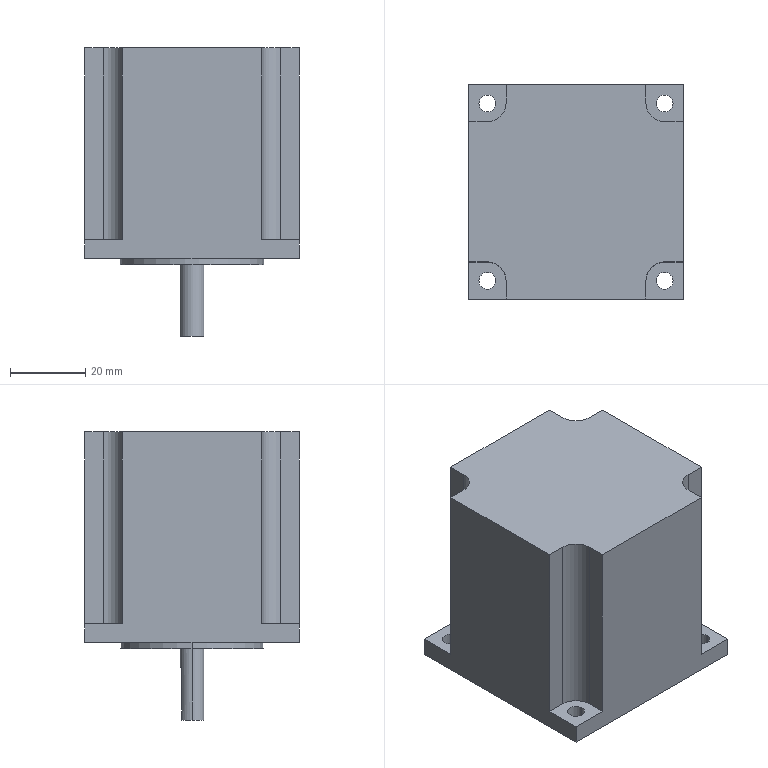Part | STEP file | Stepping motor YK57HB56-03A | 1 solid | 38 faces | box 57 x 57 x 76.6 mm | volume 165114 mm3 | plane 22 | cylinder 16 | commonest cylinder face diameters 4.5 x8 9.9 x4 6.35 x2 38.1 x2
STEP:
#1=CARTESIAN_POINT('',(-3.175,0.,-20.6));
#2=VERTEX_POINT('',#1);
#3=CARTESIAN_POINT('',(-1.71,2.675,-20.6));
#4=VERTEX_POINT('',#3);
#5=CARTESIAN_POINT('',(0.,0.,-20.6));
#6=DIRECTION('',(0.,0.,-1.));
#7=DIRECTION('',(-1.,0.,0.));
#8=AXIS2_PLACEMENT_3D('',#5,#6,#7);
#9=CIRCLE('',#8,3.175);
#10=EDGE_CURVE('',#2,#4,#9,.T.);
#11=ORIENTED_EDGE('',*,*,#10,.F.);
#12=CARTESIAN_POINT('',(-3.175,0.,-1.6));
#13=VERTEX_POINT('',#12);
#14=CARTESIAN_POINT('',(-3.175,0.,-20.6));
#15=DIRECTION('',(0.,0.,1.));
#16=VECTOR('',#15,1000.);
#17=LINE('',#14,#16);
#18=EDGE_CURVE('',#2,#13,#17,.T.);
#19=ORIENTED_EDGE('',*,*,#18,.T.);
#20=CARTESIAN_POINT('',(3.175,0.,-1.6));
#21=VERTEX_POINT('',#20);
#22=CARTESIAN_POINT('',(0.,0.,-1.6));
#23=DIRECTION('',(0.,0.,-1.));
#24=DIRECTION('',(-1.,0.,0.));
#25=AXIS2_PLACEMENT_3D('',#22,#23,#24);
#26=CIRCLE('',#25,3.175);
#27=EDGE_CURVE('',#13,#21,#26,.T.);
#28=ORIENTED_EDGE('',*,*,#27,.T.);
#29=CARTESIAN_POINT('',(3.175,0.,-20.6));
#30=VERTEX_POINT('',#29);
#31=CARTESIAN_POINT('',(3.175,0.,-20.6));
#32=DIRECTION('',(0.,0.,1.));
#33=VECTOR('',#32,1000.);
#34=LINE('',#31,#33);
#35=EDGE_CURVE('',#30,#21,#34,.T.);
#36=ORIENTED_EDGE('',*,*,#35,.F.);
#37=CARTESIAN_POINT('',(1.71,2.675,-20.6));
#38=VERTEX_POINT('',#37);
#39=CARTESIAN_POINT('',(0.,0.,-20.6));
#40=DIRECTION('',(0.,0.,-1.));
#41=DIRECTION('',(-1.,0.,0.));
#42=AXIS2_PLACEMENT_3D('',#39,#40,#41);
#43=CIRCLE('',#42,3.175);
#44=EDGE_CURVE('',#38,#30,#43,.T.);
#45=ORIENTED_EDGE('',*,*,#44,.F.);
#46=CARTESIAN_POINT('',(1.71,2.675,-6.6));
#47=VERTEX_POINT('',#46);
#48=CARTESIAN_POINT('',(1.71,2.675,-6.6));
#49=DIRECTION('',(0.,0.,-1.));
#50=VECTOR('',#49,1000.);
#51=LINE('',#48,#50);
#52=EDGE_CURVE('',#47,#38,#51,.T.);
#53=ORIENTED_EDGE('',*,*,#52,.F.);
#54=CARTESIAN_POINT('',(-1.71,2.675,-6.6));
#55=VERTEX_POINT('',#54);
#56=CARTESIAN_POINT('',(0.,0.,-6.6));
#57=DIRECTION('',(0.,0.,-1.));
#58=DIRECTION('',(-1.,0.,0.));
#59=AXIS2_PLACEMENT_3D('',#56,#57,#58);
#60=CIRCLE('',#59,3.175);
#61=EDGE_CURVE('',#55,#47,#60,.T.);
#62=ORIENTED_EDGE('',*,*,#61,.F.);
#63=CARTESIAN_POINT('',(-1.71,2.675,-6.6));
#64=DIRECTION('',(0.,0.,-1.));
#65=VECTOR('',#64,1000.);
#66=LINE('',#63,#65);
#67=EDGE_CURVE('',#55,#4,#66,.T.);
#68=ORIENTED_EDGE('',*,*,#67,.T.);
#69=EDGE_LOOP('',(#11,#19,#28,#36,#45,#53,#62,#68));
#70=FACE_OUTER_BOUND('',#69,.T.);
#71=CARTESIAN_POINT('',(0.,0.,-20.6));
#72=DIRECTION('',(0.,0.,1.));
#73=DIRECTION('',(1.,0.,0.));
#74=AXIS2_PLACEMENT_3D('',#71,#72,#73);
#75=CYLINDRICAL_SURFACE('',#74,3.175);
#76=ADVANCED_FACE('',(#70),#75,.T.);
#77=CARTESIAN_POINT('',(-19.05,0.,-1.6));
#78=VERTEX_POINT('',#77);
#79=CARTESIAN_POINT('',(19.05,0.,-1.6));
#80=VERTEX_POINT('',#79);
#81=CARTESIAN_POINT('',(0.,0.,-1.6));
#82=DIRECTION('',(0.,0.,-1.));
#83=DIRECTION('',(-1.,0.,0.));
#84=AXIS2_PLACEMENT_3D('',#81,#82,#83);
#85=CIRCLE('',#84,19.05);
#86=EDGE_CURVE('',#78,#80,#85,.T.);
#87=ORIENTED_EDGE('',*,*,#86,.F.);
#88=CARTESIAN_POINT('',(-19.05,0.,0.));
#89=VERTEX_POINT('',#88);
#90=CARTESIAN_POINT('',(-19.05,0.,-1.6));
#91=DIRECTION('',(0.,0.,1.));
#92=VECTOR('',#91,1000.);
#93=LINE('',#90,#92);
#94=EDGE_CURVE('',#78,#89,#93,.T.);
#95=ORIENTED_EDGE('',*,*,#94,.T.);
#96=CARTESIAN_POINT('',(19.05,0.,0.));
#97=VERTEX_POINT('',#96);
#98=CARTESIAN_POINT('',(0.,0.,0.));
#99=DIRECTION('',(0.,0.,-1.));
#100=DIRECTION('',(1.,0.,0.));
#101=AXIS2_PLACEMENT_3D('',#98,#99,#100);
#102=CIRCLE('',#101,19.05);
#103=EDGE_CURVE('',#89,#97,#102,.T.);
#104=ORIENTED_EDGE('',*,*,#103,.T.);
#105=CARTESIAN_POINT('',(19.05,0.,-1.6));
#106=DIRECTION('',(0.,0.,1.));
#107=VECTOR('',#106,1000.);
#108=LINE('',#105,#107);
#109=EDGE_CURVE('',#80,#97,#108,.T.);
#110=ORIENTED_EDGE('',*,*,#109,.F.);
#111=EDGE_LOOP('',(#87,#95,#104,#110));
#112=FACE_OUTER_BOUND('',#111,.T.);
#113=CARTESIAN_POINT('',(0.,0.,-1.6));
#114=DIRECTION('',(0.,0.,1.));
#115=DIRECTION('',(1.,0.,0.));
#116=AXIS2_PLACEMENT_3D('',#113,#114,#115);
#117=CYLINDRICAL_SURFACE('',#116,19.05);
#118=ADVANCED_FACE('',(#112),#117,.T.);
#119=CARTESIAN_POINT('',(21.3,-23.55,5.));
#120=VERTEX_POINT('',#119);
#121=CARTESIAN_POINT('',(25.8,-23.55,5.));
#122=VERTEX_POINT('',#121);
#123=CARTESIAN_POINT('',(23.55,-23.55,5.));
#124=DIRECTION('',(0.,0.,1.));
#125=DIRECTION('',(-1.,0.,0.));
#126=AXIS2_PLACEMENT_3D('',#123,#124,#125);
#127=CIRCLE('',#126,2.25);
#128=EDGE_CURVE('',#120,#122,#127,.T.);
#129=ORIENTED_EDGE('',*,*,#128,.T.);
#130=CARTESIAN_POINT('',(25.8,-23.55,0.));
#131=VERTEX_POINT('',#130);
#132=CARTESIAN_POINT('',(25.8,-23.55,0.));
#133=DIRECTION('',(0.,0.,-1.));
#134=VECTOR('',#133,1000.);
#135=LINE('',#132,#134);
#136=EDGE_CURVE('',#122,#131,#135,.T.);
#137=ORIENTED_EDGE('',*,*,#136,.T.);
#138=CARTESIAN_POINT('',(21.3,-23.55,0.));
#139=VERTEX_POINT('',#138);
#140=CARTESIAN_POINT('',(23.55,-23.55,0.));
#141=DIRECTION('',(0.,0.,-1.));
#142=DIRECTION('',(-1.,0.,0.));
#143=AXIS2_PLACEMENT_3D('',#140,#141,#142);
#144=CIRCLE('',#143,2.25);
#145=EDGE_CURVE('',#131,#139,#144,.T.);
#146=ORIENTED_EDGE('',*,*,#145,.T.);
#147=CARTESIAN_POINT('',(21.3,-23.55,0.));
#148=DIRECTION('',(0.,0.,-1.));
#149=VECTOR('',#148,1000.);
#150=LINE('',#147,#149);
#151=EDGE_CURVE('',#120,#139,#150,.T.);
#152=ORIENTED_EDGE('',*,*,#151,.F.);
#153=EDGE_LOOP('',(#129,#137,#146,#152));
#154=FACE_OUTER_BOUND('',#153,.T.);
#155=CARTESIAN_POINT('',(23.55,-23.55,0.));
#156=DIRECTION('',(0.,0.,-1.));
#157=DIRECTION('',(-1.,0.,0.));
#158=AXIS2_PLACEMENT_3D('',#155,#156,#157);
#159=CYLINDRICAL_SURFACE('',#158,2.25);
#160=ADVANCED_FACE('',(#154),#159,.F.);
#161=CARTESIAN_POINT('',(-25.8,-23.55,5.));
#162=VERTEX_POINT('',#161);
#163=CARTESIAN_POINT('',(-21.3,-23.55,5.));
#164=VERTEX_POINT('',#163);
#165=CARTESIAN_POINT('',(-23.55,-23.55,5.));
#166=DIRECTION('',(0.,0.,1.));
#167=DIRECTION('',(-1.,0.,0.));
#168=AXIS2_PLACEMENT_3D('',#165,#166,#167);
#169=CIRCLE('',#168,2.25);
#170=EDGE_CURVE('',#162,#164,#169,.T.);
#171=ORIENTED_EDGE('',*,*,#170,.T.);
#172=CARTESIAN_POINT('',(-21.3,-23.55,0.));
#173=VERTEX_POINT('',#172);
#174=CARTESIAN_POINT('',(-21.3,-23.55,0.));
#175=DIRECTION('',(0.,0.,-1.));
#176=VECTOR('',#175,1000.);
#177=LINE('',#174,#176);
#178=EDGE_CURVE('',#164,#173,#177,.T.);
#179=ORIENTED_EDGE('',*,*,#178,.T.);
#180=CARTESIAN_POINT('',(-25.8,-23.55,0.));
#181=VERTEX_POINT('',#180);
#182=CARTESIAN_POINT('',(-23.55,-23.55,0.));
#183=DIRECTION('',(0.,0.,-1.));
#184=DIRECTION('',(-1.,0.,0.));
#185=AXIS2_PLACEMENT_3D('',#182,#183,#184);
#186=CIRCLE('',#185,2.25);
#187=EDGE_CURVE('',#173,#181,#186,.T.);
#188=ORIENTED_EDGE('',*,*,#187,.T.);
#189=CARTESIAN_POINT('',(-25.8,-23.55,0.));
#190=DIRECTION('',(0.,0.,-1.));
#191=VECTOR('',#190,1000.);
#192=LINE('',#189,#191);
#193=EDGE_CURVE('',#162,#181,#192,.T.);
#194=ORIENTED_EDGE('',*,*,#193,.F.);
#195=EDGE_LOOP('',(#171,#179,#188,#194));
#196=FACE_OUTER_BOUND('',#195,.T.);
#197=CARTESIAN_POINT('',(-23.55,-23.55,0.));
#198=DIRECTION('',(0.,0.,-1.));
#199=DIRECTION('',(-1.,0.,0.));
#200=AXIS2_PLACEMENT_3D('',#197,#198,#199);
#201=CYLINDRICAL_SURFACE('',#200,2.25);
#202=ADVANCED_FACE('',(#196),#201,.F.);
#203=CARTESIAN_POINT('',(-25.8,23.55,5.));
#204=VERTEX_POINT('',#203);
#205=CARTESIAN_POINT('',(-21.3,23.55,5.));
#206=VERTEX_POINT('',#205);
#207=CARTESIAN_POINT('',(-23.55,23.55,5.));
#208=DIRECTION('',(0.,0.,1.));
#209=DIRECTION('',(-1.,0.,0.));
#210=AXIS2_PLACEMENT_3D('',#207,#208,#209);
#211=CIRCLE('',#210,2.25);
#212=EDGE_CURVE('',#204,#206,#211,.T.);
#213=ORIENTED_EDGE('',*,*,#212,.T.);
#214=CARTESIAN_POINT('',(-21.3,23.55,0.));
#215=VERTEX_POINT('',#214);
#216=CARTESIAN_POINT('',(-21.3,23.55,0.));
#217=DIRECTION('',(0.,0.,-1.));
#218=VECTOR('',#217,1000.);
#219=LINE('',#216,#218);
#220=EDGE_CURVE('',#206,#215,#219,.T.);
#221=ORIENTED_EDGE('',*,*,#220,.T.);
#222=CARTESIAN_POINT('',(-25.8,23.55,0.));
#223=VERTEX_POINT('',#222);
#224=CARTESIAN_POINT('',(-23.55,23.55,0.));
#225=DIRECTION('',(0.,0.,-1.));
#226=DIRECTION('',(-1.,0.,0.));
#227=AXIS2_PLACEMENT_3D('',#224,#225,#226);
#228=CIRCLE('',#227,2.25);
#229=EDGE_CURVE('',#215,#223,#228,.T.);
#230=ORIENTED_EDGE('',*,*,#229,.T.);
#231=CARTESIAN_POINT('',(-25.8,23.55,0.));
#232=DIRECTION('',(0.,0.,-1.));
#233=VECTOR('',#232,1000.);
#234=LINE('',#231,#233);
#235=EDGE_CURVE('',#204,#223,#234,.T.);
#236=ORIENTED_EDGE('',*,*,#235,.F.);
#237=EDGE_LOOP('',(#213,#221,#230,#236));
#238=FACE_OUTER_BOUND('',#237,.T.);
#239=CARTESIAN_POINT('',(-23.55,23.55,0.));
#240=DIRECTION('',(0.,0.,-1.));
#241=DIRECTION('',(-1.,0.,0.));
#242=AXIS2_PLACEMENT_3D('',#239,#240,#241);
#243=CYLINDRICAL_SURFACE('',#242,2.25);
#244=ADVANCED_FACE('',(#238),#243,.F.);
#245=CARTESIAN_POINT('',(21.3,23.55,5.));
#246=VERTEX_POINT('',#245);
#247=CARTESIAN_POINT('',(25.8,23.55,5.));
#248=VERTEX_POINT('',#247);
#249=CARTESIAN_POINT('',(23.55,23.55,5.));
#250=DIRECTION('',(0.,0.,1.));
#251=DIRECTION('',(-1.,0.,0.));
#252=AXIS2_PLACEMENT_3D('',#249,#250,#251);
#253=CIRCLE('',#252,2.25);
#254=EDGE_CURVE('',#246,#248,#253,.T.);
#255=ORIENTED_EDGE('',*,*,#254,.T.);
#256=CARTESIAN_POINT('',(25.8,23.55,0.));
#257=VERTEX_POINT('',#256);
#258=CARTESIAN_POINT('',(25.8,23.55,0.));
#259=DIRECTION('',(0.,0.,-1.));
#260=VECTOR('',#259,1000.);
#261=LINE('',#258,#260);
#262=EDGE_CURVE('',#248,#257,#261,.T.);
#263=ORIENTED_EDGE('',*,*,#262,.T.);
#264=CARTESIAN_POINT('',(21.3,23.55,0.));
#265=VERTEX_POINT('',#264);
#266=CARTESIAN_POINT('',(23.55,23.55,0.));
#267=DIRECTION('',(0.,0.,-1.));
#268=DIRECTION('',(-1.,0.,0.));
#269=AXIS2_PLACEMENT_3D('',#266,#267,#268);
#270=CIRCLE('',#269,2.25);
#271=EDGE_CURVE('',#257,#265,#270,.T.);
#272=ORIENTED_EDGE('',*,*,#271,.T.);
#273=CARTESIAN_POINT('',(21.3,23.55,0.));
#274=DIRECTION('',(0.,0.,-1.));
#275=VECTOR('',#274,1000.);
#276=LINE('',#273,#275);
#277=EDGE_CURVE('',#246,#265,#276,.T.);
#278=ORIENTED_EDGE('',*,*,#277,.F.);
#279=EDGE_LOOP('',(#255,#263,#272,#278));
#280=FACE_OUTER_BOUND('',#279,.T.);
#281=CARTESIAN_POINT('',(23.55,23.55,0.));
#282=DIRECTION('',(0.,0.,-1.));
#283=DIRECTION('',(-1.,0.,0.));
#284=AXIS2_PLACEMENT_3D('',#281,#282,#283);
#285=CYLINDRICAL_SURFACE('',#284,2.25);
#286=ADVANCED_FACE('',(#280),#285,.F.);
#287=CARTESIAN_POINT('',(-28.5,28.5,0.));
#288=VERTEX_POINT('',#287);
#289=CARTESIAN_POINT('',(-28.5,-28.5,0.));
#290=VERTEX_POINT('',#289);
#291=CARTESIAN_POINT('',(-28.5,-28.5,0.));
#292=DIRECTION('',(0.,-1.,0.));
#293=VECTOR('',#292,1000.);
#294=LINE('',#291,#293);
#295=EDGE_CURVE('',#288,#290,#294,.T.);
#296=ORIENTED_EDGE('',*,*,#295,.F.);
#297=CARTESIAN_POINT('',(28.5,28.5,0.));
#298=VERTEX_POINT('',#297);
#299=CARTESIAN_POINT('',(28.5,28.5,0.));
#300=DIRECTION('',(-1.,0.,0.));
#301=VECTOR('',#300,1000.);
#302=LINE('',#299,#301);
#303=EDGE_CURVE('',#298,#288,#302,.T.);
#304=ORIENTED_EDGE('',*,*,#303,.F.);
#305=CARTESIAN_POINT('',(28.5,-28.5,0.));
#306=VERTEX_POINT('',#305);
#307=CARTESIAN_POINT('',(28.5,-28.5,0.));
#308=DIRECTION('',(0.,1.,0.));
#309=VECTOR('',#308,1000.);
#310=LINE('',#307,#309);
#311=EDGE_CURVE('',#306,#298,#310,.T.);
#312=ORIENTED_EDGE('',*,*,#311,.F.);
#313=CARTESIAN_POINT('',(28.5,-28.5,0.));
#314=DIRECTION('',(1.,0.,0.));
#315=VECTOR('',#314,1000.);
#316=LINE('',#313,#315);
#317=EDGE_CURVE('',#290,#306,#316,.T.);
#318=ORIENTED_EDGE('',*,*,#317,.F.);
#319=EDGE_LOOP('',(#296,#304,#312,#318));
#320=FACE_OUTER_BOUND('',#319,.T.);
#321=CARTESIAN_POINT('',(23.55,23.55,0.));
#322=DIRECTION('',(0.,0.,-1.));
#323=DIRECTION('',(-1.,0.,0.));
#324=AXIS2_PLACEMENT_3D('',#321,#322,#323);
#325=CIRCLE('',#324,2.25);
#326=EDGE_CURVE('',#265,#257,#325,.T.);
#327=ORIENTED_EDGE('',*,*,#326,.F.);
#328=ORIENTED_EDGE('',*,*,#271,.F.);
#329=EDGE_LOOP('',(#327,#328));
#330=FACE_BOUND('',#329,.T.);
#331=CARTESIAN_POINT('',(-23.55,23.55,0.));
#332=DIRECTION('',(0.,0.,-1.));
#333=DIRECTION('',(-1.,0.,0.));
#334=AXIS2_PLACEMENT_3D('',#331,#332,#333);
#335=CIRCLE('',#334,2.25);
#336=EDGE_CURVE('',#223,#215,#335,.T.);
#337=ORIENTED_EDGE('',*,*,#336,.F.);
#338=ORIENTED_EDGE('',*,*,#229,.F.);
#339=EDGE_LOOP('',(#337,#338));
#340=FACE_BOUND('',#339,.T.);
#341=CARTESIAN_POINT('',(-23.55,-23.55,0.));
#342=DIRECTION('',(0.,0.,-1.));
#343=DIRECTION('',(-1.,0.,0.));
#344=AXIS2_PLACEMENT_3D('',#341,#342,#343);
#345=CIRCLE('',#344,2.25);
#346=EDGE_CURVE('',#181,#173,#345,.T.);
#347=ORIENTED_EDGE('',*,*,#346,.F.);
#348=ORIENTED_EDGE('',*,*,#187,.F.);
#349=EDGE_LOOP('',(#347,#348));
#350=FACE_BOUND('',#349,.T.);
#351=CARTESIAN_POINT('',(23.55,-23.55,0.));
#352=DIRECTION('',(0.,0.,-1.));
#353=DIRECTION('',(-1.,0.,0.));
#354=AXIS2_PLACEMENT_3D('',#351,#352,#353);
#355=CIRCLE('',#354,2.25);
#356=EDGE_CURVE('',#139,#131,#355,.T.);
#357=ORIENTED_EDGE('',*,*,#356,.F.);
#358=ORIENTED_EDGE('',*,*,#145,.F.);
#359=EDGE_LOOP('',(#357,#358));
#360=FACE_BOUND('',#359,.T.);
#361=CARTESIAN_POINT('',(0.,0.,0.));
#362=DIRECTION('',(0.,0.,-1.));
#363=DIRECTION('',(1.,0.,0.));
#364=AXIS2_PLACEMENT_3D('',#361,#362,#363);
#365=CIRCLE('',#364,19.05);
#366=EDGE_CURVE('',#97,#89,#365,.T.);
#367=ORIENTED_EDGE('',*,*,#366,.F.);
#368=ORIENTED_EDGE('',*,*,#103,.F.);
#369=EDGE_LOOP('',(#367,#368));
#370=FACE_BOUND('',#369,.T.);
#371=CARTESIAN_POINT('',(-28.5,28.5,0.));
#372=DIRECTION('',(0.,0.,1.));
#373=DIRECTION('',(1.,0.,0.));
#374=AXIS2_PLACEMENT_3D('',#371,#372,#373);
#375=PLANE('',#374);
#376=ADVANCED_FACE('',(#320,#330,#340,#350,#360,#370),#375,.F.);
#377=CARTESIAN_POINT('',(-28.5,-28.5,5.));
#378=VERTEX_POINT('',#377);
#379=CARTESIAN_POINT('',(-28.5,-18.6,5.));
#380=VERTEX_POINT('',#379);
#381=CARTESIAN_POINT('',(-28.5,-18.6,5.));
#382=DIRECTION('',(0.,1.,0.));
#383=VECTOR('',#382,1000.);
#384=LINE('',#381,#383);
#385=EDGE_CURVE('',#378,#380,#384,.T.);
#386=ORIENTED_EDGE('',*,*,#385,.T.);
#387=CARTESIAN_POINT('',(-28.5,-18.6,56.));
#388=VERTEX_POINT('',#387);
#389=CARTESIAN_POINT('',(-28.5,-18.6,56.));
#390=DIRECTION('',(0.,0.,-1.));
#391=VECTOR('',#390,1000.);
#392=LINE('',#389,#391);
#393=EDGE_CURVE('',#388,#380,#392,.T.);
#394=ORIENTED_EDGE('',*,*,#393,.F.);
#395=CARTESIAN_POINT('',(-28.5,18.6,56.));
#396=VERTEX_POINT('',#395);
#397=CARTESIAN_POINT('',(-28.5,-28.5,56.));
#398=DIRECTION('',(0.,-1.,0.));
#399=VECTOR('',#398,1000.);
#400=LINE('',#397,#399);
#401=EDGE_CURVE('',#396,#388,#400,.T.);
#402=ORIENTED_EDGE('',*,*,#401,.F.);
#403=CARTESIAN_POINT('',(-28.5,18.6,5.));
#404=VERTEX_POINT('',#403);
#405=CARTESIAN_POINT('',(-28.5,18.6,56.));
#406=DIRECTION('',(0.,0.,-1.));
#407=VECTOR('',#406,1000.);
#408=LINE('',#405,#407);
#409=EDGE_CURVE('',#396,#404,#408,.T.);
#410=ORIENTED_EDGE('',*,*,#409,.T.);
#411=CARTESIAN_POINT('',(-28.5,28.5,5.));
#412=VERTEX_POINT('',#411);
#413=CARTESIAN_POINT('',(-28.5,28.5,5.));
#414=DIRECTION('',(0.,1.,0.));
#415=VECTOR('',#414,1000.);
#416=LINE('',#413,#415);
#417=EDGE_CURVE('',#404,#412,#416,.T.);
#418=ORIENTED_EDGE('',*,*,#417,.T.);
#419=CARTESIAN_POINT('',(-28.5,28.5,56.));
#420=DIRECTION('',(0.,0.,-1.));
#421=VECTOR('',#420,1000.);
#422=LINE('',#419,#421);
#423=EDGE_CURVE('',#412,#288,#422,.T.);
#424=ORIENTED_EDGE('',*,*,#423,.T.);
#425=ORIENTED_EDGE('',*,*,#295,.T.);
#426=CARTESIAN_POINT('',(-28.5,-28.5,56.));
#427=DIRECTION('',(0.,0.,-1.));
#428=VECTOR('',#427,1000.);
#429=LINE('',#426,#428);
#430=EDGE_CURVE('',#378,#290,#429,.T.);
#431=ORIENTED_EDGE('',*,*,#430,.F.);
#432=EDGE_LOOP('',(#386,#394,#402,#410,#418,#424,#425,#431));
#433=FACE_OUTER_BOUND('',#432,.T.);
#434=CARTESIAN_POINT('',(-28.5,-28.5,56.));
#435=DIRECTION('',(1.,0.,0.));
#436=DIRECTION('',(0.,0.,-1.));
#437=AXIS2_PLACEMENT_3D('',#434,#435,#436);
#438=PLANE('',#437);
#439=ADVANCED_FACE('',(#433),#438,.F.);
#440=CARTESIAN_POINT('',(28.5,-28.5,5.));
#441=VERTEX_POINT('',#440);
#442=CARTESIAN_POINT('',(18.6,-28.5,5.));
#443=VERTEX_POINT('',#442);
#444=CARTESIAN_POINT('',(18.6,-28.5,5.));
#445=DIRECTION('',(-1.,0.,0.));
#446=VECTOR('',#445,1000.);
#447=LINE('',#444,#446);
#448=EDGE_CURVE('',#441,#443,#447,.T.);
#449=ORIENTED_EDGE('',*,*,#448,.T.);
#450=CARTESIAN_POINT('',(18.6,-28.5,56.));
#451=VERTEX_POINT('',#450);
#452=CARTESIAN_POINT('',(18.6,-28.5,56.));
#453=DIRECTION('',(0.,0.,-1.));
#454=VECTOR('',#453,1000.);
#455=LINE('',#452,#454);
#456=EDGE_CURVE('',#451,#443,#455,.T.);
#457=ORIENTED_EDGE('',*,*,#456,.F.);
#458=CARTESIAN_POINT('',(-18.6,-28.5,56.));
#459=VERTEX_POINT('',#458);
#460=CARTESIAN_POINT('',(28.5,-28.5,56.));
#461=DIRECTION('',(1.,0.,0.));
#462=VECTOR('',#461,1000.);
#463=LINE('',#460,#462);
#464=EDGE_CURVE('',#459,#451,#463,.T.);
#465=ORIENTED_EDGE('',*,*,#464,.F.);
#466=CARTESIAN_POINT('',(-18.6,-28.5,5.));
#467=VERTEX_POINT('',#466);
#468=CARTESIAN_POINT('',(-18.6,-28.5,56.));
#469=DIRECTION('',(0.,0.,-1.));
#470=VECTOR('',#469,1000.);
#471=LINE('',#468,#470);
#472=EDGE_CURVE('',#459,#467,#471,.T.);
#473=ORIENTED_EDGE('',*,*,#472,.T.);
#474=CARTESIAN_POINT('',(-28.5,-28.5,5.));
#475=DIRECTION('',(-1.,0.,0.));
#476=VECTOR('',#475,1000.);
#477=LINE('',#474,#476);
#478=EDGE_CURVE('',#467,#378,#477,.T.);
#479=ORIENTED_EDGE('',*,*,#478,.T.);
#480=ORIENTED_EDGE('',*,*,#430,.T.);
#481=ORIENTED_EDGE('',*,*,#317,.T.);
#482=CARTESIAN_POINT('',(28.5,-28.5,56.));
#483=DIRECTION('',(0.,0.,-1.));
#484=VECTOR('',#483,1000.);
#485=LINE('',#482,#484);
#486=EDGE_CURVE('',#441,#306,#485,.T.);
#487=ORIENTED_EDGE('',*,*,#486,.F.);
#488=EDGE_LOOP('',(#449,#457,#465,#473,#479,#480,#481,#487));
#489=FACE_OUTER_BOUND('',#488,.T.);
#490=CARTESIAN_POINT('',(28.5,-28.5,56.));
#491=DIRECTION('',(0.,1.,0.));
#492=DIRECTION('',(-1.,0.,0.));
#493=AXIS2_PLACEMENT_3D('',#490,#491,#492);
#494=PLANE('',#493);
#495=ADVANCED_FACE('',(#489),#494,.F.);
#496=CARTESIAN_POINT('',(28.5,-18.6,56.));
#497=VERTEX_POINT('',#496);
#498=CARTESIAN_POINT('',(28.5,18.6,56.));
#499=VERTEX_POINT('',#498);
#500=CARTESIAN_POINT('',(28.5,-28.5,56.));
#501=DIRECTION('',(0.,1.,0.));
#502=VECTOR('',#501,1000.);
#503=LINE('',#500,#502);
#504=EDGE_CURVE('',#497,#499,#503,.T.);
#505=ORIENTED_EDGE('',*,*,#504,.F.);
#506=CARTESIAN_POINT('',(28.5,-18.6,5.));
#507=VERTEX_POINT('',#506);
#508=CARTESIAN_POINT('',(28.5,-18.6,56.));
#509=DIRECTION('',(0.,0.,-1.));
#510=VECTOR('',#509,1000.);
#511=LINE('',#508,#510);
#512=EDGE_CURVE('',#497,#507,#511,.T.);
#513=ORIENTED_EDGE('',*,*,#512,.T.);
#514=CARTESIAN_POINT('',(28.5,-28.5,5.));
#515=DIRECTION('',(0.,-1.,0.));
#516=VECTOR('',#515,1000.);
#517=LINE('',#514,#516);
#518=EDGE_CURVE('',#507,#441,#517,.T.);
#519=ORIENTED_EDGE('',*,*,#518,.T.);
#520=ORIENTED_EDGE('',*,*,#486,.T.);
#521=ORIENTED_EDGE('',*,*,#311,.T.);
#522=CARTESIAN_POINT('',(28.5,28.5,5.));
#523=VERTEX_POINT('',#522);
#524=CARTESIAN_POINT('',(28.5,28.5,56.));
#525=DIRECTION('',(0.,0.,-1.));
#526=VECTOR('',#525,1000.);
#527=LINE('',#524,#526);
#528=EDGE_CURVE('',#523,#298,#527,.T.);
#529=ORIENTED_EDGE('',*,*,#528,.F.);
#530=CARTESIAN_POINT('',(28.5,18.6,5.));
#531=VERTEX_POINT('',#530);
#532=CARTESIAN_POINT('',(28.5,18.6,5.));
#533=DIRECTION('',(0.,-1.,0.));
#534=VECTOR('',#533,1000.);
#535=LINE('',#532,#534);
#536=EDGE_CURVE('',#523,#531,#535,.T.);
#537=ORIENTED_EDGE('',*,*,#536,.T.);
#538=CARTESIAN_POINT('',(28.5,18.6,56.));
#539=DIRECTION('',(0.,0.,-1.));
#540=VECTOR('',#539,1000.);
#541=LINE('',#538,#540);
#542=EDGE_CURVE('',#499,#531,#541,.T.);
#543=ORIENTED_EDGE('',*,*,#542,.F.);
#544=EDGE_LOOP('',(#505,#513,#519,#520,#521,#529,#537,#543));
#545=FACE_OUTER_BOUND('',#544,.T.);
#546=CARTESIAN_POINT('',(28.5,-28.5,56.));
#547=DIRECTION('',(-1.,0.,0.));
#548=DIRECTION('',(0.,0.,1.));
#549=AXIS2_PLACEMENT_3D('',#546,#547,#548);
#550=PLANE('',#549);
#551=ADVANCED_FACE('',(#545),#550,.F.);
#552=CARTESIAN_POINT('',(-18.6,28.5,5.));
#553=VERTEX_POINT('',#552);
#554=CARTESIAN_POINT('',(-18.6,28.5,5.));
#555=DIRECTION('',(1.,0.,0.));
#556=VECTOR('',#555,1000.);
#557=LINE('',#554,#556);
#558=EDGE_CURVE('',#412,#553,#557,.T.);
#559=ORIENTED_EDGE('',*,*,#558,.T.);
#560=CARTESIAN_POINT('',(-18.6,28.5,56.));
#561=VERTEX_POINT('',#560);
#562=CARTESIAN_POINT('',(-18.6,28.5,56.));
#563=DIRECTION('',(0.,0.,-1.));
#564=VECTOR('',#563,1000.);
#565=LINE('',#562,#564);
#566=EDGE_CURVE('',#561,#553,#565,.T.);
#567=ORIENTED_EDGE('',*,*,#566,.F.);
#568=CARTESIAN_POINT('',(18.6,28.5,56.));
#569=VERTEX_POINT('',#568);
#570=CARTESIAN_POINT('',(28.5,28.5,56.));
#571=DIRECTION('',(-1.,0.,0.));
#572=VECTOR('',#571,1000.);
#573=LINE('',#570,#572);
#574=EDGE_CURVE('',#569,#561,#573,.T.);
#575=ORIENTED_EDGE('',*,*,#574,.F.);
#576=CARTESIAN_POINT('',(18.6,28.5,5.));
#577=VERTEX_POINT('',#576);
#578=CARTESIAN_POINT('',(18.6,28.5,56.));
#579=DIRECTION('',(0.,0.,-1.));
#580=VECTOR('',#579,1000.);
#581=LINE('',#578,#580);
#582=EDGE_CURVE('',#569,#577,#581,.T.);
#583=ORIENTED_EDGE('',*,*,#582,.T.);
#584=CARTESIAN_POINT('',(28.5,28.5,5.));
#585=DIRECTION('',(1.,0.,0.));
#586=VECTOR('',#585,1000.);
#587=LINE('',#584,#586);
#588=EDGE_CURVE('',#577,#523,#587,.T.);
#589=ORIENTED_EDGE('',*,*,#588,.T.);
#590=ORIENTED_EDGE('',*,*,#528,.T.);
#591=ORIENTED_EDGE('',*,*,#303,.T.);
#592=ORIENTED_EDGE('',*,*,#423,.F.);
#593=EDGE_LOOP('',(#559,#567,#575,#583,#589,#590,#591,#592));
#594=FACE_OUTER_BOUND('',#593,.T.);
#595=CARTESIAN_POINT('',(28.5,28.5,56.));
#596=DIRECTION('',(0.,-1.,0.));
#597=DIRECTION('',(1.,0.,0.));
#598=AXIS2_PLACEMENT_3D('',#595,#596,#597);
#599=PLANE('',#598);
#600=ADVANCED_FACE('',(#594),#599,.F.);
#601=CARTESIAN_POINT('',(23.55,-18.6,56.));
#602=VERTEX_POINT('',#601);
#603=CARTESIAN_POINT('',(28.5,-18.6,56.));
#604=DIRECTION('',(1.,0.,0.));
#605=VECTOR('',#604,1000.);
#606=LINE('',#603,#605);
#607=EDGE_CURVE('',#602,#497,#606,.T.);
#608=ORIENTED_EDGE('',*,*,#607,.T.);
#609=ORIENTED_EDGE('',*,*,#504,.T.);
#610=CARTESIAN_POINT('',(23.55,18.6,56.));
#611=VERTEX_POINT('',#610);
#612=CARTESIAN_POINT('',(23.55,18.6,56.));
#613=DIRECTION('',(-1.,0.,0.));
#614=VECTOR('',#613,1000.);
#615=LINE('',#612,#614);
#616=EDGE_CURVE('',#499,#611,#615,.T.);
#617=ORIENTED_EDGE('',*,*,#616,.T.);
#618=CARTESIAN_POINT('',(18.6,23.55,56.));
#619=VERTEX_POINT('',#618);
#620=CARTESIAN_POINT('',(23.55,23.55,56.));
#621=DIRECTION('',(0.,0.,-1.));
#622=DIRECTION('',(-1.,0.,0.));
#623=AXIS2_PLACEMENT_3D('',#620,#621,#622);
#624=CIRCLE('',#623,4.95);
#625=EDGE_CURVE('',#611,#619,#624,.T.);
#626=ORIENTED_EDGE('',*,*,#625,.T.);
#627=CARTESIAN_POINT('',(18.6,28.5,56.));
#628=DIRECTION('',(0.,1.,0.));
#629=VECTOR('',#628,1000.);
#630=LINE('',#627,#629);
#631=EDGE_CURVE('',#619,#569,#630,.T.);
#632=ORIENTED_EDGE('',*,*,#631,.T.);
#633=ORIENTED_EDGE('',*,*,#574,.T.);
#634=CARTESIAN_POINT('',(-18.6,23.55,56.));
#635=VERTEX_POINT('',#634);
#636=CARTESIAN_POINT('',(-18.6,23.55,56.));
#637=DIRECTION('',(0.,-1.,0.));
#638=VECTOR('',#637,1000.);
#639=LINE('',#636,#638);
#640=EDGE_CURVE('',#561,#635,#639,.T.);
#641=ORIENTED_EDGE('',*,*,#640,.T.);
#642=CARTESIAN_POINT('',(-23.55,18.6,56.));
#643=VERTEX_POINT('',#642);
#644=CARTESIAN_POINT('',(-23.55,23.55,56.));
#645=DIRECTION('',(0.,0.,-1.));
#646=DIRECTION('',(0.,-1.,0.));
#647=AXIS2_PLACEMENT_3D('',#644,#645,#646);
#648=CIRCLE('',#647,4.95);
#649=EDGE_CURVE('',#635,#643,#648,.T.);
#650=ORIENTED_EDGE('',*,*,#649,.T.);
#651=CARTESIAN_POINT('',(-28.5,18.6,56.));
#652=DIRECTION('',(-1.,0.,0.));
#653=VECTOR('',#652,1000.);
#654=LINE('',#651,#653);
#655=EDGE_CURVE('',#643,#396,#654,.T.);
#656=ORIENTED_EDGE('',*,*,#655,.T.);
#657=ORIENTED_EDGE('',*,*,#401,.T.);
#658=CARTESIAN_POINT('',(-23.55,-18.6,56.));
#659=VERTEX_POINT('',#658);
#660=CARTESIAN_POINT('',(-23.55,-18.6,56.));
#661=DIRECTION('',(1.,0.,0.));
#662=VECTOR('',#661,1000.);
#663=LINE('',#660,#662);
#664=EDGE_CURVE('',#388,#659,#663,.T.);
#665=ORIENTED_EDGE('',*,*,#664,.T.);
#666=CARTESIAN_POINT('',(-18.6,-23.55,56.));
#667=VERTEX_POINT('',#666);
#668=CARTESIAN_POINT('',(-23.55,-23.55,56.));
#669=DIRECTION('',(0.,0.,-1.));
#670=DIRECTION('',(1.,0.,0.));
#671=AXIS2_PLACEMENT_3D('',#668,#669,#670);
#672=CIRCLE('',#671,4.95);
#673=EDGE_CURVE('',#659,#667,#672,.T.);
#674=ORIENTED_EDGE('',*,*,#673,.T.);
#675=CARTESIAN_POINT('',(-18.6,-28.5,56.));
#676=DIRECTION('',(0.,-1.,0.));
#677=VECTOR('',#676,1000.);
#678=LINE('',#675,#677);
#679=EDGE_CURVE('',#667,#459,#678,.T.);
#680=ORIENTED_EDGE('',*,*,#679,.T.);
#681=ORIENTED_EDGE('',*,*,#464,.T.);
#682=CARTESIAN_POINT('',(18.6,-23.55,56.));
#683=VERTEX_POINT('',#682);
#684=CARTESIAN_POINT('',(18.6,-23.55,56.));
#685=DIRECTION('',(0.,1.,0.));
#686=VECTOR('',#685,1000.);
#687=LINE('',#684,#686);
#688=EDGE_CURVE('',#451,#683,#687,.T.);
#689=ORIENTED_EDGE('',*,*,#688,.T.);
#690=CARTESIAN_POINT('',(23.55,-23.55,56.));
#691=DIRECTION('',(0.,0.,-1.));
#692=DIRECTION('',(0.,1.,0.));
#693=AXIS2_PLACEMENT_3D('',#690,#691,#692);
#694=CIRCLE('',#693,4.95);
#695=EDGE_CURVE('',#683,#602,#694,.T.);
#696=ORIENTED_EDGE('',*,*,#695,.T.);
#697=EDGE_LOOP('',(#608,#609,#617,#626,#632,#633,#641,#650,#656,#657,#665,#674,#680,#681,#689,#696));
#698=FACE_OUTER_BOUND('',#697,.T.);
#699=CARTESIAN_POINT('',(-28.5,28.5,56.));
#700=DIRECTION('',(0.,0.,1.));
#701=DIRECTION('',(1.,0.,0.));
#702=AXIS2_PLACEMENT_3D('',#699,#700,#701);
#703=PLANE('',#702);
#704=ADVANCED_FACE('',(#698),#703,.T.);
#705=ORIENTED_EDGE('',*,*,#262,.F.);
#706=CARTESIAN_POINT('',(23.55,23.55,5.));
#707=DIRECTION('',(0.,0.,1.));
#708=DIRECTION('',(-1.,0.,0.));
#709=AXIS2_PLACEMENT_3D('',#706,#707,#708);
#710=CIRCLE('',#709,2.25);
#711=EDGE_CURVE('',#248,#246,#710,.T.);
#712=ORIENTED_EDGE('',*,*,#711,.T.);
#713=ORIENTED_EDGE('',*,*,#277,.T.);
#714=ORIENTED_EDGE('',*,*,#326,.T.);
#715=EDGE_LOOP('',(#705,#712,#713,#714));
#716=FACE_OUTER_BOUND('',#715,.T.);
#717=CARTESIAN_POINT('',(23.55,23.55,0.));
#718=DIRECTION('',(0.,0.,-1.));
#719=DIRECTION('',(-1.,0.,0.));
#720=AXIS2_PLACEMENT_3D('',#717,#718,#719);
#721=CYLINDRICAL_SURFACE('',#720,2.25);
#722=ADVANCED_FACE('',(#716),#721,.F.);
#723=ORIENTED_EDGE('',*,*,#220,.F.);
#724=CARTESIAN_POINT('',(-23.55,23.55,5.));
#725=DIRECTION('',(0.,0.,1.));
#726=DIRECTION('',(-1.,0.,0.));
#727=AXIS2_PLACEMENT_3D('',#724,#725,#726);
#728=CIRCLE('',#727,2.25);
#729=EDGE_CURVE('',#206,#204,#728,.T.);
#730=ORIENTED_EDGE('',*,*,#729,.T.);
#731=ORIENTED_EDGE('',*,*,#235,.T.);
#732=ORIENTED_EDGE('',*,*,#336,.T.);
#733=EDGE_LOOP('',(#723,#730,#731,#732));
#734=FACE_OUTER_BOUND('',#733,.T.);
#735=CARTESIAN_POINT('',(-23.55,23.55,0.));
#736=DIRECTION('',(0.,0.,-1.));
#737=DIRECTION('',(-1.,0.,0.));
#738=AXIS2_PLACEMENT_3D('',#735,#736,#737);
#739=CYLINDRICAL_SURFACE('',#738,2.25);
#740=ADVANCED_FACE('',(#734),#739,.F.);
#741=ORIENTED_EDGE('',*,*,#178,.F.);
#742=CARTESIAN_POINT('',(-23.55,-23.55,5.));
#743=DIRECTION('',(0.,0.,1.));
#744=DIRECTION('',(-1.,0.,0.));
#745=AXIS2_PLACEMENT_3D('',#742,#743,#744);
#746=CIRCLE('',#745,2.25);
#747=EDGE_CURVE('',#164,#162,#746,.T.);
#748=ORIENTED_EDGE('',*,*,#747,.T.);
#749=ORIENTED_EDGE('',*,*,#193,.T.);
#750=ORIENTED_EDGE('',*,*,#346,.T.);
#751=EDGE_LOOP('',(#741,#748,#749,#750));
#752=FACE_OUTER_BOUND('',#751,.T.);
#753=CARTESIAN_POINT('',(-23.55,-23.55,0.));
#754=DIRECTION('',(0.,0.,-1.));
#755=DIRECTION('',(-1.,0.,0.));
#756=AXIS2_PLACEMENT_3D('',#753,#754,#755);
#757=CYLINDRICAL_SURFACE('',#756,2.25);
#758=ADVANCED_FACE('',(#752),#757,.F.);
#759=ORIENTED_EDGE('',*,*,#136,.F.);
#760=CARTESIAN_POINT('',(23.55,-23.55,5.));
#761=DIRECTION('',(0.,0.,1.));
#762=DIRECTION('',(-1.,0.,0.));
#763=AXIS2_PLACEMENT_3D('',#760,#761,#762);
#764=CIRCLE('',#763,2.25);
#765=EDGE_CURVE('',#122,#120,#764,.T.);
#766=ORIENTED_EDGE('',*,*,#765,.T.);
#767=ORIENTED_EDGE('',*,*,#151,.T.);
#768=ORIENTED_EDGE('',*,*,#356,.T.);
#769=EDGE_LOOP('',(#759,#766,#767,#768));
#770=FACE_OUTER_BOUND('',#769,.T.);
#771=CARTESIAN_POINT('',(23.55,-23.55,0.));
#772=DIRECTION('',(0.,0.,-1.));
#773=DIRECTION('',(-1.,0.,0.));
#774=AXIS2_PLACEMENT_3D('',#771,#772,#773);
#775=CYLINDRICAL_SURFACE('',#774,2.25);
#776=ADVANCED_FACE('',(#770),#775,.F.);
#777=CARTESIAN_POINT('',(0.,0.,-1.6));
#778=DIRECTION('',(0.,0.,-1.));
#779=DIRECTION('',(-1.,0.,0.));
#780=AXIS2_PLACEMENT_3D('',#777,#778,#779);
#781=CIRCLE('',#780,19.05);
#782=EDGE_CURVE('',#80,#78,#781,.T.);
#783=ORIENTED_EDGE('',*,*,#782,.T.);
#784=ORIENTED_EDGE('',*,*,#86,.T.);
#785=EDGE_LOOP('',(#783,#784));
#786=FACE_OUTER_BOUND('',#785,.T.);
#787=CARTESIAN_POINT('',(0.,0.,-1.6));
#788=DIRECTION('',(0.,0.,-1.));
#789=DIRECTION('',(-1.,0.,0.));
#790=AXIS2_PLACEMENT_3D('',#787,#788,#789);
#791=CIRCLE('',#790,3.175);
#792=EDGE_CURVE('',#21,#13,#791,.T.);
#793=ORIENTED_EDGE('',*,*,#792,.F.);
#794=ORIENTED_EDGE('',*,*,#27,.F.);
#795=EDGE_LOOP('',(#793,#794));
#796=FACE_BOUND('',#795,.T.);
#797=CARTESIAN_POINT('',(0.,0.,-1.6));
#798=DIRECTION('',(0.,0.,-1.));
#799=DIRECTION('',(-1.,0.,0.));
#800=AXIS2_PLACEMENT_3D('',#797,#798,#799);
#801=PLANE('',#800);
#802=ADVANCED_FACE('',(#786,#796),#801,.T.);
#803=ORIENTED_EDGE('',*,*,#94,.F.);
#804=ORIENTED_EDGE('',*,*,#782,.F.);
#805=ORIENTED_EDGE('',*,*,#109,.T.);
#806=ORIENTED_EDGE('',*,*,#366,.T.);
#807=EDGE_LOOP('',(#803,#804,#805,#806));
#808=FACE_OUTER_BOUND('',#807,.T.);
#809=CARTESIAN_POINT('',(0.,0.,-1.6));
#810=DIRECTION('',(0.,0.,1.));
#811=DIRECTION('',(1.,0.,0.));
#812=AXIS2_PLACEMENT_3D('',#809,#810,#811);
#813=CYLINDRICAL_SURFACE('',#812,19.05);
#814=ADVANCED_FACE('',(#808),#813,.T.);
#815=CARTESIAN_POINT('',(1.71,2.675,-20.6));
#816=DIRECTION('',(-1.,0.,0.));
#817=VECTOR('',#816,1000.);
#818=LINE('',#815,#817);
#819=EDGE_CURVE('',#38,#4,#818,.T.);
#820=ORIENTED_EDGE('',*,*,#819,.F.);
#821=ORIENTED_EDGE('',*,*,#44,.T.);
#822=CARTESIAN_POINT('',(0.,0.,-20.6));
#823=DIRECTION('',(0.,0.,-1.));
#824=DIRECTION('',(-1.,0.,0.));
#825=AXIS2_PLACEMENT_3D('',#822,#823,#824);
#826=CIRCLE('',#825,3.175);
#827=EDGE_CURVE('',#30,#2,#826,.T.);
#828=ORIENTED_EDGE('',*,*,#827,.T.);
#829=ORIENTED_EDGE('',*,*,#10,.T.);
#830=EDGE_LOOP('',(#820,#821,#828,#829));
#831=FACE_OUTER_BOUND('',#830,.T.);
#832=CARTESIAN_POINT('',(0.,0.,-20.6));
#833=DIRECTION('',(0.,0.,-1.));
#834=DIRECTION('',(-1.,0.,0.));
#835=AXIS2_PLACEMENT_3D('',#832,#833,#834);
#836=PLANE('',#835);
#837=ADVANCED_FACE('',(#831),#836,.T.);
#838=ORIENTED_EDGE('',*,*,#18,.F.);
#839=ORIENTED_EDGE('',*,*,#827,.F.);
#840=ORIENTED_EDGE('',*,*,#35,.T.);
#841=ORIENTED_EDGE('',*,*,#792,.T.);
#842=EDGE_LOOP('',(#838,#839,#840,#841));
#843=FACE_OUTER_BOUND('',#842,.T.);
#844=CARTESIAN_POINT('',(0.,0.,-20.6));
#845=DIRECTION('',(0.,0.,1.));
#846=DIRECTION('',(1.,0.,0.));
#847=AXIS2_PLACEMENT_3D('',#844,#845,#846);
#848=CYLINDRICAL_SURFACE('',#847,3.175);
#849=ADVANCED_FACE('',(#843),#848,.T.);
#850=ORIENTED_EDGE('',*,*,#536,.F.);
#851=ORIENTED_EDGE('',*,*,#588,.F.);
#852=CARTESIAN_POINT('',(18.6,23.55,5.));
#853=VERTEX_POINT('',#852);
#854=CARTESIAN_POINT('',(18.6,28.5,5.));
#855=DIRECTION('',(0.,1.,0.));
#856=VECTOR('',#855,1000.);
#857=LINE('',#854,#856);
#858=EDGE_CURVE('',#853,#577,#857,.T.);
#859=ORIENTED_EDGE('',*,*,#858,.F.);
#860=CARTESIAN_POINT('',(23.55,18.6,5.));
#861=VERTEX_POINT('',#860);
#862=CARTESIAN_POINT('',(23.55,23.55,5.));
#863=DIRECTION('',(0.,0.,-1.));
#864=DIRECTION('',(-1.,0.,0.));
#865=AXIS2_PLACEMENT_3D('',#862,#863,#864);
#866=CIRCLE('',#865,4.95);
#867=EDGE_CURVE('',#861,#853,#866,.T.);
#868=ORIENTED_EDGE('',*,*,#867,.F.);
#869=CARTESIAN_POINT('',(23.55,18.6,5.));
#870=DIRECTION('',(-1.,0.,0.));
#871=VECTOR('',#870,1000.);
#872=LINE('',#869,#871);
#873=EDGE_CURVE('',#531,#861,#872,.T.);
#874=ORIENTED_EDGE('',*,*,#873,.F.);
#875=EDGE_LOOP('',(#850,#851,#859,#868,#874));
#876=FACE_OUTER_BOUND('',#875,.T.);
#877=ORIENTED_EDGE('',*,*,#254,.F.);
#878=ORIENTED_EDGE('',*,*,#711,.F.);
#879=EDGE_LOOP('',(#877,#878));
#880=FACE_BOUND('',#879,.T.);
#881=CARTESIAN_POINT('',(23.55,23.55,5.));
#882=DIRECTION('',(0.,0.,-1.));
#883=DIRECTION('',(-1.,0.,0.));
#884=AXIS2_PLACEMENT_3D('',#881,#882,#883);
#885=PLANE('',#884);
#886=ADVANCED_FACE('',(#876,#880),#885,.F.);
#887=ORIENTED_EDGE('',*,*,#858,.T.);
#888=ORIENTED_EDGE('',*,*,#582,.F.);
#889=ORIENTED_EDGE('',*,*,#631,.F.);
#890=CARTESIAN_POINT('',(18.6,23.55,56.));
#891=DIRECTION('',(0.,0.,-1.));
#892=VECTOR('',#891,1000.);
#893=LINE('',#890,#892);
#894=EDGE_CURVE('',#619,#853,#893,.T.);
#895=ORIENTED_EDGE('',*,*,#894,.T.);
#896=EDGE_LOOP('',(#887,#888,#889,#895));
#897=FACE_OUTER_BOUND('',#896,.T.);
#898=CARTESIAN_POINT('',(18.6,28.5,56.));
#899=DIRECTION('',(-1.,0.,0.));
#900=DIRECTION('',(0.,0.,1.));
#901=AXIS2_PLACEMENT_3D('',#898,#899,#900);
#902=PLANE('',#901);
#903=ADVANCED_FACE('',(#897),#902,.F.);
#904=ORIENTED_EDGE('',*,*,#867,.T.);
#905=ORIENTED_EDGE('',*,*,#894,.F.);
#906=ORIENTED_EDGE('',*,*,#625,.F.);
#907=CARTESIAN_POINT('',(23.55,18.6,56.));
#908=DIRECTION('',(0.,0.,-1.));
#909=VECTOR('',#908,1000.);
#910=LINE('',#907,#909);
#911=EDGE_CURVE('',#611,#861,#910,.T.);
#912=ORIENTED_EDGE('',*,*,#911,.T.);
#913=EDGE_LOOP('',(#904,#905,#906,#912));
#914=FACE_OUTER_BOUND('',#913,.T.);
#915=CARTESIAN_POINT('',(23.55,23.55,56.));
#916=DIRECTION('',(0.,0.,-1.));
#917=DIRECTION('',(-1.,0.,0.));
#918=AXIS2_PLACEMENT_3D('',#915,#916,#917);
#919=CYLINDRICAL_SURFACE('',#918,4.95);
#920=ADVANCED_FACE('',(#914),#919,.F.);
#921=ORIENTED_EDGE('',*,*,#873,.T.);
#922=ORIENTED_EDGE('',*,*,#911,.F.);
#923=ORIENTED_EDGE('',*,*,#616,.F.);
#924=ORIENTED_EDGE('',*,*,#542,.T.);
#925=EDGE_LOOP('',(#921,#922,#923,#924));
#926=FACE_OUTER_BOUND('',#925,.T.);
#927=CARTESIAN_POINT('',(23.55,18.6,56.));
#928=DIRECTION('',(0.,-1.,0.));
#929=DIRECTION('',(0.,0.,-1.));
#930=AXIS2_PLACEMENT_3D('',#927,#928,#929);
#931=PLANE('',#930);
#932=ADVANCED_FACE('',(#926),#931,.F.);
#933=ORIENTED_EDGE('',*,*,#558,.F.);
#934=ORIENTED_EDGE('',*,*,#417,.F.);
#935=CARTESIAN_POINT('',(-23.55,18.6,5.));
#936=VERTEX_POINT('',#935);
#937=CARTESIAN_POINT('',(-28.5,18.6,5.));
#938=DIRECTION('',(-1.,0.,0.));
#939=VECTOR('',#938,1000.);
#940=LINE('',#937,#939);
#941=EDGE_CURVE('',#936,#404,#940,.T.);
#942=ORIENTED_EDGE('',*,*,#941,.F.);
#943=CARTESIAN_POINT('',(-18.6,23.55,5.));
#944=VERTEX_POINT('',#943);
#945=CARTESIAN_POINT('',(-23.55,23.55,5.));
#946=DIRECTION('',(0.,0.,-1.));
#947=DIRECTION('',(0.,-1.,0.));
#948=AXIS2_PLACEMENT_3D('',#945,#946,#947);
#949=CIRCLE('',#948,4.95);
#950=EDGE_CURVE('',#944,#936,#949,.T.);
#951=ORIENTED_EDGE('',*,*,#950,.F.);
#952=CARTESIAN_POINT('',(-18.6,23.55,5.));
#953=DIRECTION('',(0.,-1.,0.));
#954=VECTOR('',#953,1000.);
#955=LINE('',#952,#954);
#956=EDGE_CURVE('',#553,#944,#955,.T.);
#957=ORIENTED_EDGE('',*,*,#956,.F.);
#958=EDGE_LOOP('',(#933,#934,#942,#951,#957));
#959=FACE_OUTER_BOUND('',#958,.T.);
#960=ORIENTED_EDGE('',*,*,#212,.F.);
#961=ORIENTED_EDGE('',*,*,#729,.F.);
#962=EDGE_LOOP('',(#960,#961));
#963=FACE_BOUND('',#962,.T.);
#964=CARTESIAN_POINT('',(-23.55,23.55,5.));
#965=DIRECTION('',(0.,0.,-1.));
#966=DIRECTION('',(0.,-1.,0.));
#967=AXIS2_PLACEMENT_3D('',#964,#965,#966);
#968=PLANE('',#967);
#969=ADVANCED_FACE('',(#959,#963),#968,.F.);
#970=ORIENTED_EDGE('',*,*,#941,.T.);
#971=ORIENTED_EDGE('',*,*,#409,.F.);
#972=ORIENTED_EDGE('',*,*,#655,.F.);
#973=CARTESIAN_POINT('',(-23.55,18.6,56.));
#974=DIRECTION('',(0.,0.,-1.));
#975=VECTOR('',#974,1000.);
#976=LINE('',#973,#975);
#977=EDGE_CURVE('',#643,#936,#976,.T.);
#978=ORIENTED_EDGE('',*,*,#977,.T.);
#979=EDGE_LOOP('',(#970,#971,#972,#978));
#980=FACE_OUTER_BOUND('',#979,.T.);
#981=CARTESIAN_POINT('',(-28.5,18.6,56.));
#982=DIRECTION('',(0.,-1.,0.));
#983=DIRECTION('',(1.,0.,0.));
#984=AXIS2_PLACEMENT_3D('',#981,#982,#983);
#985=PLANE('',#984);
#986=ADVANCED_FACE('',(#980),#985,.F.);
#987=ORIENTED_EDGE('',*,*,#950,.T.);
#988=ORIENTED_EDGE('',*,*,#977,.F.);
#989=ORIENTED_EDGE('',*,*,#649,.F.);
#990=CARTESIAN_POINT('',(-18.6,23.55,56.));
#991=DIRECTION('',(0.,0.,-1.));
#992=VECTOR('',#991,1000.);
#993=LINE('',#990,#992);
#994=EDGE_CURVE('',#635,#944,#993,.T.);
#995=ORIENTED_EDGE('',*,*,#994,.T.);
#996=EDGE_LOOP('',(#987,#988,#989,#995));
#997=FACE_OUTER_BOUND('',#996,.T.);
#998=CARTESIAN_POINT('',(-23.55,23.55,56.));
#999=DIRECTION('',(0.,0.,-1.));
#1000=DIRECTION('',(-1.,0.,0.));
#1001=AXIS2_PLACEMENT_3D('',#998,#999,#1000);
#1002=CYLINDRICAL_SURFACE('',#1001,4.95);
#1003=ADVANCED_FACE('',(#997),#1002,.F.);
#1004=ORIENTED_EDGE('',*,*,#956,.T.);
#1005=ORIENTED_EDGE('',*,*,#994,.F.);
#1006=ORIENTED_EDGE('',*,*,#640,.F.);
#1007=ORIENTED_EDGE('',*,*,#566,.T.);
#1008=EDGE_LOOP('',(#1004,#1005,#1006,#1007));
#1009=FACE_OUTER_BOUND('',#1008,.T.);
#1010=CARTESIAN_POINT('',(-18.6,23.55,56.));
#1011=DIRECTION('',(1.,0.,0.));
#1012=DIRECTION('',(0.,1.,0.));
#1013=AXIS2_PLACEMENT_3D('',#1010,#1011,#1012);
#1014=PLANE('',#1013);
#1015=ADVANCED_FACE('',(#1009),#1014,.F.);
#1016=ORIENTED_EDGE('',*,*,#385,.F.);
#1017=ORIENTED_EDGE('',*,*,#478,.F.);
#1018=CARTESIAN_POINT('',(-18.6,-23.55,5.));
#1019=VERTEX_POINT('',#1018);
#1020=CARTESIAN_POINT('',(-18.6,-28.5,5.));
#1021=DIRECTION('',(0.,-1.,0.));
#1022=VECTOR('',#1021,1000.);
#1023=LINE('',#1020,#1022);
#1024=EDGE_CURVE('',#1019,#467,#1023,.T.);
#1025=ORIENTED_EDGE('',*,*,#1024,.F.);
#1026=CARTESIAN_POINT('',(-23.55,-18.6,5.));
#1027=VERTEX_POINT('',#1026);
#1028=CARTESIAN_POINT('',(-23.55,-23.55,5.));
#1029=DIRECTION('',(0.,0.,-1.));
#1030=DIRECTION('',(1.,0.,0.));
#1031=AXIS2_PLACEMENT_3D('',#1028,#1029,#1030);
#1032=CIRCLE('',#1031,4.95);
#1033=EDGE_CURVE('',#1027,#1019,#1032,.T.);
#1034=ORIENTED_EDGE('',*,*,#1033,.F.);
#1035=CARTESIAN_POINT('',(-23.55,-18.6,5.));
#1036=DIRECTION('',(1.,0.,0.));
#1037=VECTOR('',#1036,1000.);
#1038=LINE('',#1035,#1037);
#1039=EDGE_CURVE('',#380,#1027,#1038,.T.);
#1040=ORIENTED_EDGE('',*,*,#1039,.F.);
#1041=EDGE_LOOP('',(#1016,#1017,#1025,#1034,#1040));
#1042=FACE_OUTER_BOUND('',#1041,.T.);
#1043=ORIENTED_EDGE('',*,*,#170,.F.);
#1044=ORIENTED_EDGE('',*,*,#747,.F.);
#1045=EDGE_LOOP('',(#1043,#1044));
#1046=FACE_BOUND('',#1045,.T.);
#1047=CARTESIAN_POINT('',(-23.55,-23.55,5.));
#1048=DIRECTION('',(0.,0.,-1.));
#1049=DIRECTION('',(1.,0.,0.));
#1050=AXIS2_PLACEMENT_3D('',#1047,#1048,#1049);
#1051=PLANE('',#1050);
#1052=ADVANCED_FACE('',(#1042,#1046),#1051,.F.);
#1053=ORIENTED_EDGE('',*,*,#1024,.T.);
#1054=ORIENTED_EDGE('',*,*,#472,.F.);
#1055=ORIENTED_EDGE('',*,*,#679,.F.);
#1056=CARTESIAN_POINT('',(-18.6,-23.55,56.));
#1057=DIRECTION('',(0.,0.,-1.));
#1058=VECTOR('',#1057,1000.);
#1059=LINE('',#1056,#1058);
#1060=EDGE_CURVE('',#667,#1019,#1059,.T.);
#1061=ORIENTED_EDGE('',*,*,#1060,.T.);
#1062=EDGE_LOOP('',(#1053,#1054,#1055,#1061));
#1063=FACE_OUTER_BOUND('',#1062,.T.);
#1064=CARTESIAN_POINT('',(-18.6,-28.5,56.));
#1065=DIRECTION('',(1.,0.,0.));
#1066=DIRECTION('',(0.,0.,-1.));
#1067=AXIS2_PLACEMENT_3D('',#1064,#1065,#1066);
#1068=PLANE('',#1067);
#1069=ADVANCED_FACE('',(#1063),#1068,.F.);
#1070=ORIENTED_EDGE('',*,*,#1033,.T.);
#1071=ORIENTED_EDGE('',*,*,#1060,.F.);
#1072=ORIENTED_EDGE('',*,*,#673,.F.);
#1073=CARTESIAN_POINT('',(-23.55,-18.6,56.));
#1074=DIRECTION('',(0.,0.,-1.));
#1075=VECTOR('',#1074,1000.);
#1076=LINE('',#1073,#1075);
#1077=EDGE_CURVE('',#659,#1027,#1076,.T.);
#1078=ORIENTED_EDGE('',*,*,#1077,.T.);
#1079=EDGE_LOOP('',(#1070,#1071,#1072,#1078));
#1080=FACE_OUTER_BOUND('',#1079,.T.);
#1081=CARTESIAN_POINT('',(-23.55,-23.55,56.));
#1082=DIRECTION('',(0.,0.,-1.));
#1083=DIRECTION('',(-1.,0.,0.));
#1084=AXIS2_PLACEMENT_3D('',#1081,#1082,#1083);
#1085=CYLINDRICAL_SURFACE('',#1084,4.95);
#1086=ADVANCED_FACE('',(#1080),#1085,.F.);
#1087=ORIENTED_EDGE('',*,*,#1039,.T.);
#1088=ORIENTED_EDGE('',*,*,#1077,.F.);
#1089=ORIENTED_EDGE('',*,*,#664,.F.);
#1090=ORIENTED_EDGE('',*,*,#393,.T.);
#1091=EDGE_LOOP('',(#1087,#1088,#1089,#1090));
#1092=FACE_OUTER_BOUND('',#1091,.T.);
#1093=CARTESIAN_POINT('',(-23.55,-18.6,56.));
#1094=DIRECTION('',(0.,1.,0.));
#1095=DIRECTION('',(0.,0.,1.));
#1096=AXIS2_PLACEMENT_3D('',#1093,#1094,#1095);
#1097=PLANE('',#1096);
#1098=ADVANCED_FACE('',(#1092),#1097,.F.);
#1099=ORIENTED_EDGE('',*,*,#448,.F.);
#1100=ORIENTED_EDGE('',*,*,#518,.F.);
#1101=CARTESIAN_POINT('',(23.55,-18.6,5.));
#1102=VERTEX_POINT('',#1101);
#1103=CARTESIAN_POINT('',(28.5,-18.6,5.));
#1104=DIRECTION('',(1.,0.,0.));
#1105=VECTOR('',#1104,1000.);
#1106=LINE('',#1103,#1105);
#1107=EDGE_CURVE('',#1102,#507,#1106,.T.);
#1108=ORIENTED_EDGE('',*,*,#1107,.F.);
#1109=CARTESIAN_POINT('',(18.6,-23.55,5.));
#1110=VERTEX_POINT('',#1109);
#1111=CARTESIAN_POINT('',(23.55,-23.55,5.));
#1112=DIRECTION('',(0.,0.,-1.));
#1113=DIRECTION('',(0.,1.,0.));
#1114=AXIS2_PLACEMENT_3D('',#1111,#1112,#1113);
#1115=CIRCLE('',#1114,4.95);
#1116=EDGE_CURVE('',#1110,#1102,#1115,.T.);
#1117=ORIENTED_EDGE('',*,*,#1116,.F.);
#1118=CARTESIAN_POINT('',(18.6,-23.55,5.));
#1119=DIRECTION('',(0.,1.,0.));
#1120=VECTOR('',#1119,1000.);
#1121=LINE('',#1118,#1120);
#1122=EDGE_CURVE('',#443,#1110,#1121,.T.);
#1123=ORIENTED_EDGE('',*,*,#1122,.F.);
#1124=EDGE_LOOP('',(#1099,#1100,#1108,#1117,#1123));
#1125=FACE_OUTER_BOUND('',#1124,.T.);
#1126=ORIENTED_EDGE('',*,*,#128,.F.);
#1127=ORIENTED_EDGE('',*,*,#765,.F.);
#1128=EDGE_LOOP('',(#1126,#1127));
#1129=FACE_BOUND('',#1128,.T.);
#1130=CARTESIAN_POINT('',(23.55,-23.55,5.));
#1131=DIRECTION('',(0.,0.,-1.));
#1132=DIRECTION('',(0.,1.,0.));
#1133=AXIS2_PLACEMENT_3D('',#1130,#1131,#1132);
#1134=PLANE('',#1133);
#1135=ADVANCED_FACE('',(#1125,#1129),#1134,.F.);
#1136=ORIENTED_EDGE('',*,*,#1107,.T.);
#1137=ORIENTED_EDGE('',*,*,#512,.F.);
#1138=ORIENTED_EDGE('',*,*,#607,.F.);
#1139=CARTESIAN_POINT('',(23.55,-18.6,56.));
#1140=DIRECTION('',(0.,0.,-1.));
#1141=VECTOR('',#1140,1000.);
#1142=LINE('',#1139,#1141);
#1143=EDGE_CURVE('',#602,#1102,#1142,.T.);
#1144=ORIENTED_EDGE('',*,*,#1143,.T.);
#1145=EDGE_LOOP('',(#1136,#1137,#1138,#1144));
#1146=FACE_OUTER_BOUND('',#1145,.T.);
#1147=CARTESIAN_POINT('',(28.5,-18.6,56.));
#1148=DIRECTION('',(0.,1.,0.));
#1149=DIRECTION('',(-1.,0.,0.));
#1150=AXIS2_PLACEMENT_3D('',#1147,#1148,#1149);
#1151=PLANE('',#1150);
#1152=ADVANCED_FACE('',(#1146),#1151,.F.);
#1153=ORIENTED_EDGE('',*,*,#1116,.T.);
#1154=ORIENTED_EDGE('',*,*,#1143,.F.);
#1155=ORIENTED_EDGE('',*,*,#695,.F.);
#1156=CARTESIAN_POINT('',(18.6,-23.55,56.));
#1157=DIRECTION('',(0.,0.,-1.));
#1158=VECTOR('',#1157,1000.);
#1159=LINE('',#1156,#1158);
#1160=EDGE_CURVE('',#683,#1110,#1159,.T.);
#1161=ORIENTED_EDGE('',*,*,#1160,.T.);
#1162=EDGE_LOOP('',(#1153,#1154,#1155,#1161));
#1163=FACE_OUTER_BOUND('',#1162,.T.);
#1164=CARTESIAN_POINT('',(23.55,-23.55,56.));
#1165=DIRECTION('',(0.,0.,-1.));
#1166=DIRECTION('',(-1.,0.,0.));
#1167=AXIS2_PLACEMENT_3D('',#1164,#1165,#1166);
#1168=CYLINDRICAL_SURFACE('',#1167,4.95);
#1169=ADVANCED_FACE('',(#1163),#1168,.F.);
#1170=ORIENTED_EDGE('',*,*,#1122,.T.);
#1171=ORIENTED_EDGE('',*,*,#1160,.F.);
#1172=ORIENTED_EDGE('',*,*,#688,.F.);
#1173=ORIENTED_EDGE('',*,*,#456,.T.);
#1174=EDGE_LOOP('',(#1170,#1171,#1172,#1173));
#1175=FACE_OUTER_BOUND('',#1174,.T.);
#1176=CARTESIAN_POINT('',(18.6,-23.55,56.));
#1177=DIRECTION('',(-1.,0.,0.));
#1178=DIRECTION('',(0.,-1.,0.));
#1179=AXIS2_PLACEMENT_3D('',#1176,#1177,#1178);
#1180=PLANE('',#1179);
#1181=ADVANCED_FACE('',(#1175),#1180,.F.);
#1182=ORIENTED_EDGE('',*,*,#819,.T.);
#1183=ORIENTED_EDGE('',*,*,#67,.F.);
#1184=CARTESIAN_POINT('',(1.71,2.675,-6.6));
#1185=DIRECTION('',(-1.,0.,0.));
#1186=VECTOR('',#1185,1000.);
#1187=LINE('',#1184,#1186);
#1188=EDGE_CURVE('',#47,#55,#1187,.T.);
#1189=ORIENTED_EDGE('',*,*,#1188,.F.);
#1190=ORIENTED_EDGE('',*,*,#52,.T.);
#1191=EDGE_LOOP('',(#1182,#1183,#1189,#1190));
#1192=FACE_OUTER_BOUND('',#1191,.T.);
#1193=CARTESIAN_POINT('',(1.71,2.675,-6.6));
#1194=DIRECTION('',(0.,-1.,0.));
#1195=DIRECTION('',(0.,0.,-1.));
#1196=AXIS2_PLACEMENT_3D('',#1193,#1194,#1195);
#1197=PLANE('',#1196);
#1198=ADVANCED_FACE('',(#1192),#1197,.F.);
#1199=ORIENTED_EDGE('',*,*,#61,.T.);
#1200=ORIENTED_EDGE('',*,*,#1188,.T.);
#1201=EDGE_LOOP('',(#1199,#1200));
#1202=FACE_OUTER_BOUND('',#1201,.T.);
#1203=CARTESIAN_POINT('',(0.,0.,-6.6));
#1204=DIRECTION('',(0.,0.,-1.));
#1205=DIRECTION('',(-1.,0.,0.));
#1206=AXIS2_PLACEMENT_3D('',#1203,#1204,#1205);
#1207=PLANE('',#1206);
#1208=ADVANCED_FACE('',(#1202),#1207,.T.);
#1209=CLOSED_SHELL('',(#76,#118,#160,#202,#244,#286,#376,#439,#495,#551,#600,#704,#722,#740,#758,#776,#802,#814,#837,#849,#886,#903,#920,#932,#969,#986,#1003,#1015,#1052,#1069,#1086,#1098,#1135,#1152,#1169,#1181,#1198,#1208));
#1210=MANIFOLD_SOLID_BREP('',#1209);
#1211=CARTESIAN_POINT('',(0.,0.,0.));
#1212=DIRECTION('',(0.,0.,1.));
#1213=DIRECTION('',(1.,0.,0.));
#1214=AXIS2_PLACEMENT_3D('',#1211,#1212,#1213);
#1215=(LENGTH_UNIT()NAMED_UNIT(*)SI_UNIT(.MILLI.,.METRE.));
#1216=UNCERTAINTY_MEASURE_WITH_UNIT(LENGTH_MEASURE(0.00001),#1215,'','');
#1217=(NAMED_UNIT(*)PLANE_ANGLE_UNIT()SI_UNIT($,.RADIAN.));
#1218=(NAMED_UNIT(*)SI_UNIT($,.STERADIAN.)SOLID_ANGLE_UNIT());
#1219=(GEOMETRIC_REPRESENTATION_CONTEXT(3)GLOBAL_UNCERTAINTY_ASSIGNED_CONTEXT((#1216))GLOBAL_UNIT_ASSIGNED_CONTEXT((#1215,#1217,#1218))REPRESENTATION_CONTEXT('',''));
#1220=ADVANCED_BREP_SHAPE_REPRESENTATION('',(#1210,#1214),#1219);